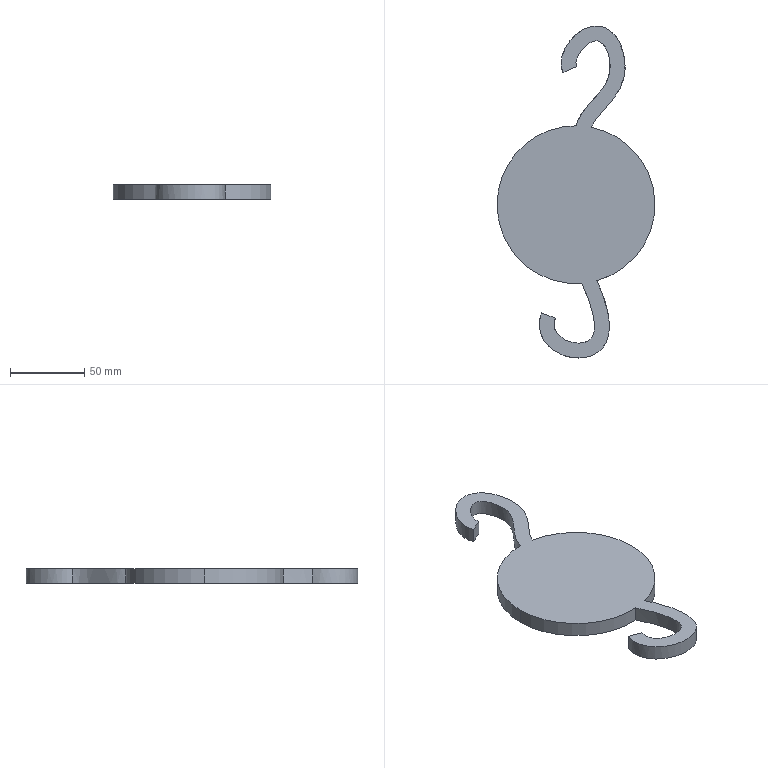Part | STEP file | Spring scale | 1 solid | 11 faces | box 106.116 x 223.189 x 10 mm | volume 107592 mm3 | plane 4 | spline 4 | cylinder 3 | commonest cylinder face diameters 106.116 x3
STEP:
#1=CARTESIAN_POINT('',(0.,0.,0.));
#2=DIRECTION('',(0.,0.,1.));
#3=DIRECTION('',(1.,0.,0.));
#4=AXIS2_PLACEMENT_3D('',#1,#2,#3);
#5=CARTESIAN_POINT('',(-53.422,-92.835,10.));
#6=VERTEX_POINT('',#5);
#7=CARTESIAN_POINT('',(3.465,-145.754,10.));
#8=VERTEX_POINT('',#7);
#9=CARTESIAN_POINT('',(-0.3636,-92.835,10.));
#10=DIRECTION('',(0.,0.,1.));
#11=DIRECTION('',(-1.,0.,0.));
#12=AXIS2_PLACEMENT_3D('',#9,#10,#11);
#13=CIRCLE('',#12,53.058);
#14=CARTESIAN_POINT('',(-0.3636,-92.835,10.));
#15=DIRECTION('',(0.,0.,-1.));
#16=DIRECTION('',(-1.,0.,0.));
#17=AXIS2_PLACEMENT_3D('',#14,#15,#16);
#18=CYLINDRICAL_SURFACE('',#17,53.058);
#19=CARTESIAN_POINT('',(6.283,0.));
#20=DIRECTION('',(-1.,0.));
#21=VECTOR('',#20,1.);
#22=LINE('',#19,#21);
#23=(GEOMETRIC_REPRESENTATION_CONTEXT(2)PARAMETRIC_REPRESENTATION_CONTEXT()REPRESENTATION_CONTEXT('',''));
#24=DEFINITIONAL_REPRESENTATION('',(#22),#23);
#25=PCURVE('',#18,#24);
#26=CARTESIAN_POINT('',(22.563,-1.634,10.));
#27=DIRECTION('',(0.,0.,1.));
#28=DIRECTION('',(1.,0.,0.));
#29=AXIS2_PLACEMENT_3D('',#26,#27,#28);
#30=PLANE('',#29);
#31=CARTESIAN_POINT('',(-22.927,-91.2));
#32=DIRECTION('',(-1.,0.));
#33=AXIS2_PLACEMENT_2D('',#31,#32);
#34=CIRCLE('',#33,53.058);
#35=(GEOMETRIC_REPRESENTATION_CONTEXT(2)PARAMETRIC_REPRESENTATION_CONTEXT()REPRESENTATION_CONTEXT('',''));
#36=DEFINITIONAL_REPRESENTATION('',(#34),#35);
#37=PCURVE('',#30,#36);
#38=SURFACE_CURVE('',#13,(#25,#37),.PCURVE_S1.);
#39=EDGE_CURVE('',#6,#8,#38,.T.);
#40=ORIENTED_EDGE('',*,*,#39,.F.);
#41=CARTESIAN_POINT('',(-53.422,-92.835,0.));
#42=VERTEX_POINT('',#41);
#43=CARTESIAN_POINT('',(-53.422,-92.835,10.));
#44=DIRECTION('',(0.,0.,-1.));
#45=VECTOR('',#44,1.);
#46=LINE('',#43,#45);
#47=CARTESIAN_POINT('',(6.283,0.));
#48=DIRECTION('',(0.,1.));
#49=VECTOR('',#48,1.);
#50=LINE('',#47,#49);
#51=(GEOMETRIC_REPRESENTATION_CONTEXT(2)PARAMETRIC_REPRESENTATION_CONTEXT()REPRESENTATION_CONTEXT('',''));
#52=DEFINITIONAL_REPRESENTATION('',(#50),#51);
#53=PCURVE('',#18,#52);
#54=CARTESIAN_POINT('',(-0.3636,-92.835,10.));
#55=DIRECTION('',(0.,0.,-1.));
#56=DIRECTION('',(-1.,0.,0.));
#57=AXIS2_PLACEMENT_3D('',#54,#55,#56);
#58=CYLINDRICAL_SURFACE('',#57,53.058);
#59=CARTESIAN_POINT('',(0.,0.));
#60=DIRECTION('',(0.,1.));
#61=VECTOR('',#60,1.);
#62=LINE('',#59,#61);
#63=(GEOMETRIC_REPRESENTATION_CONTEXT(2)PARAMETRIC_REPRESENTATION_CONTEXT()REPRESENTATION_CONTEXT('',''));
#64=DEFINITIONAL_REPRESENTATION('',(#62),#63);
#65=PCURVE('',#58,#64);
#66=SURFACE_CURVE('',#46,(#53,#65),.PCURVE_S1.);
#67=EDGE_CURVE('',#6,#42,#66,.T.);
#68=ORIENTED_EDGE('',*,*,#67,.T.);
#69=CARTESIAN_POINT('',(3.465,-145.754,0.));
#70=VERTEX_POINT('',#69);
#71=CARTESIAN_POINT('',(-0.3636,-92.835,0.));
#72=DIRECTION('',(0.,0.,1.));
#73=DIRECTION('',(-1.,0.,0.));
#74=AXIS2_PLACEMENT_3D('',#71,#72,#73);
#75=CIRCLE('',#74,53.058);
#76=CARTESIAN_POINT('',(6.283,10.));
#77=DIRECTION('',(-1.,0.));
#78=VECTOR('',#77,1.);
#79=LINE('',#76,#78);
#80=(GEOMETRIC_REPRESENTATION_CONTEXT(2)PARAMETRIC_REPRESENTATION_CONTEXT()REPRESENTATION_CONTEXT('',''));
#81=DEFINITIONAL_REPRESENTATION('',(#79),#80);
#82=PCURVE('',#18,#81);
#83=CARTESIAN_POINT('',(22.563,-1.634,0.));
#84=DIRECTION('',(0.,0.,1.));
#85=DIRECTION('',(1.,0.,0.));
#86=AXIS2_PLACEMENT_3D('',#83,#84,#85);
#87=PLANE('',#86);
#88=CARTESIAN_POINT('',(-22.927,-91.2));
#89=DIRECTION('',(-1.,0.));
#90=AXIS2_PLACEMENT_2D('',#88,#89);
#91=CIRCLE('',#90,53.058);
#92=(GEOMETRIC_REPRESENTATION_CONTEXT(2)PARAMETRIC_REPRESENTATION_CONTEXT()REPRESENTATION_CONTEXT('',''));
#93=DEFINITIONAL_REPRESENTATION('',(#91),#92);
#94=PCURVE('',#87,#93);
#95=SURFACE_CURVE('',#75,(#82,#94),.PCURVE_S1.);
#96=EDGE_CURVE('',#42,#70,#95,.T.);
#97=ORIENTED_EDGE('',*,*,#96,.T.);
#98=CARTESIAN_POINT('',(3.465,-145.754,5.));
#99=DIRECTION('',(0.,0.,1.));
#100=VECTOR('',#99,1.);
#101=LINE('',#98,#100);
#102=CARTESIAN_POINT('',(4.64,5.));
#103=DIRECTION('',(0.,-1.));
#104=VECTOR('',#103,1.);
#105=LINE('',#102,#104);
#106=(GEOMETRIC_REPRESENTATION_CONTEXT(2)PARAMETRIC_REPRESENTATION_CONTEXT()REPRESENTATION_CONTEXT('',''));
#107=DEFINITIONAL_REPRESENTATION('',(#105),#106);
#108=PCURVE('',#18,#107);
#109=CARTESIAN_POINT('',(3.465,-145.754,10.));
#110=CARTESIAN_POINT('',(3.465,-145.754,0.));
#111=CARTESIAN_POINT('',(3.905,-146.754,10.));
#112=CARTESIAN_POINT('',(3.905,-146.754,0.));
#113=CARTESIAN_POINT('',(6.76,-153.123,10.));
#114=CARTESIAN_POINT('',(6.76,-153.123,0.));
#115=CARTESIAN_POINT('',(11.768,-164.41,10.));
#116=CARTESIAN_POINT('',(11.768,-164.41,0.));
#117=CARTESIAN_POINT('',(14.007,-193.617,10.));
#118=CARTESIAN_POINT('',(14.007,-193.617,0.));
#119=CARTESIAN_POINT('',(-19.503,-183.153,10.));
#120=CARTESIAN_POINT('',(-19.503,-183.153,0.));
#121=CARTESIAN_POINT('',(-14.276,-169.124,10.));
#122=CARTESIAN_POINT('',(-14.276,-169.124,0.));
#123=B_SPLINE_SURFACE_WITH_KNOTS('',3,1,((#109,#110),(#111,#112),(#113,#114),(#115,#116),(#117,#118),(#119,#120),(#121,#122)),.UNSPECIFIED.,.F.,.F.,.F.,(4,1,1,1,4),(2,2),(0.1276,0.1688,0.393,0.6051,1.),(0.,1.),.UNSPECIFIED.);
#124=CARTESIAN_POINT('',(0.1276,1.));
#125=CARTESIAN_POINT('',(0.1276,0.));
#126=B_SPLINE_CURVE_WITH_KNOTS('',1,(#124,#125),.UNSPECIFIED.,.F.,.F.,(2,2),(-5.,5.),.PIECEWISE_BEZIER_KNOTS.);
#127=(GEOMETRIC_REPRESENTATION_CONTEXT(2)PARAMETRIC_REPRESENTATION_CONTEXT()REPRESENTATION_CONTEXT('',''));
#128=DEFINITIONAL_REPRESENTATION('',(#126),#127);
#129=PCURVE('',#123,#128);
#130=SURFACE_CURVE('',#101,(#108,#129),.PCURVE_S1.);
#131=EDGE_CURVE('',#70,#8,#130,.T.);
#132=ORIENTED_EDGE('',*,*,#131,.T.);
#133=EDGE_LOOP('',(#40,#68,#97,#132));
#134=FACE_BOUND('',#133,.T.);
#135=ADVANCED_FACE('',(#134),#18,.T.);
#136=CARTESIAN_POINT('',(9.947,-40.788,10.));
#137=VERTEX_POINT('',#136);
#138=CARTESIAN_POINT('',(-9.171,-3.986,10.));
#139=VERTEX_POINT('',#138);
#140=CARTESIAN_POINT('',(9.947,-40.788,10.));
#141=CARTESIAN_POINT('',(9.973,-40.716,10.));
#142=CARTESIAN_POINT('',(10.186,-40.135,10.));
#143=CARTESIAN_POINT('',(10.896,-38.523,10.));
#144=CARTESIAN_POINT('',(12.625,-35.777,10.));
#145=CARTESIAN_POINT('',(15.676,-32.099,10.));
#146=CARTESIAN_POINT('',(19.453,-28.011,10.));
#147=CARTESIAN_POINT('',(23.604,-23.334,10.));
#148=CARTESIAN_POINT('',(27.701,-17.742,10.));
#149=CARTESIAN_POINT('',(31.119,-10.826,10.));
#150=CARTESIAN_POINT('',(32.629,-3.898,10.));
#151=CARTESIAN_POINT('',(32.657,2.114,10.));
#152=CARTESIAN_POINT('',(32.128,6.58,10.));
#153=CARTESIAN_POINT('',(31.095,11.,10.));
#154=CARTESIAN_POINT('',(29.509,15.321,10.));
#155=CARTESIAN_POINT('',(27.223,19.502,10.));
#156=CARTESIAN_POINT('',(24.407,22.836,10.));
#157=CARTESIAN_POINT('',(21.236,25.171,10.));
#158=CARTESIAN_POINT('',(18.804,26.334,10.));
#159=CARTESIAN_POINT('',(16.636,26.962,10.));
#160=CARTESIAN_POINT('',(14.328,27.351,10.));
#161=CARTESIAN_POINT('',(11.527,27.321,10.));
#162=CARTESIAN_POINT('',(8.59,26.717,10.));
#163=CARTESIAN_POINT('',(5.149,25.439,10.));
#164=CARTESIAN_POINT('',(1.56,23.266,10.));
#165=CARTESIAN_POINT('',(-2.066,20.114,10.));
#166=CARTESIAN_POINT('',(-5.162,16.517,10.));
#167=CARTESIAN_POINT('',(-7.732,12.507,10.));
#168=CARTESIAN_POINT('',(-9.364,8.756,10.));
#169=CARTESIAN_POINT('',(-10.205,5.348,10.));
#170=CARTESIAN_POINT('',(-10.504,2.526,10.));
#171=CARTESIAN_POINT('',(-10.332,-0.09537,10.));
#172=CARTESIAN_POINT('',(-9.821,-2.3,10.));
#173=CARTESIAN_POINT('',(-9.408,-3.44,10.));
#174=CARTESIAN_POINT('',(-9.171,-3.986,10.));
#175=B_SPLINE_CURVE_WITH_KNOTS('',3,(#140,#141,#142,#143,#144,#145,#146,#147,#148,#149,#150,#151,#152,#153,#154,#155,#156,#157,#158,#159,#160,#161,#162,#163,#164,#165,#166,#167,#168,#169,#170,#171,#172,#173,#174),.UNSPECIFIED.,.F.,.F.,(4,1,1,1,1,1,1,1,1,1,1,1,1,1,1,1,1,1,1,1,1,1,1,1,1,1,1,1,1,1,1,1,4),(0.,0.0005756,0.004611,0.01268,0.02075,0.02883,0.0369,0.04497,0.05304,0.06111,0.06515,0.06919,0.07322,0.07726,0.08129,0.08533,0.08735,0.08936,0.09037,0.09138,0.0934,0.09542,0.09744,0.1015,0.1055,0.1095,0.1136,0.1176,0.1196,0.1217,0.1237,0.1247,0.1257),.UNSPECIFIED.);
#176=CARTESIAN_POINT('',(-12.616,-39.154));
#177=CARTESIAN_POINT('',(-12.59,-39.082));
#178=CARTESIAN_POINT('',(-12.378,-38.501));
#179=CARTESIAN_POINT('',(-11.667,-36.889));
#180=CARTESIAN_POINT('',(-9.938,-34.143));
#181=CARTESIAN_POINT('',(-6.887,-30.465));
#182=CARTESIAN_POINT('',(-3.11,-26.376));
#183=CARTESIAN_POINT('',(1.04,-21.7));
#184=CARTESIAN_POINT('',(5.137,-16.108));
#185=CARTESIAN_POINT('',(8.556,-9.191));
#186=CARTESIAN_POINT('',(10.065,-2.264));
#187=CARTESIAN_POINT('',(10.093,3.749));
#188=CARTESIAN_POINT('',(9.565,8.214));
#189=CARTESIAN_POINT('',(8.532,12.635));
#190=CARTESIAN_POINT('',(6.946,16.955));
#191=CARTESIAN_POINT('',(4.66,21.136));
#192=CARTESIAN_POINT('',(1.844,24.47));
#193=CARTESIAN_POINT('',(-1.328,26.806));
#194=CARTESIAN_POINT('',(-3.759,27.969));
#195=CARTESIAN_POINT('',(-5.927,28.596));
#196=CARTESIAN_POINT('',(-8.235,28.985));
#197=CARTESIAN_POINT('',(-11.036,28.955));
#198=CARTESIAN_POINT('',(-13.973,28.351));
#199=CARTESIAN_POINT('',(-17.415,27.073));
#200=CARTESIAN_POINT('',(-21.003,24.9));
#201=CARTESIAN_POINT('',(-24.629,21.749));
#202=CARTESIAN_POINT('',(-27.726,18.151));
#203=CARTESIAN_POINT('',(-30.296,14.141));
#204=CARTESIAN_POINT('',(-31.927,10.39));
#205=CARTESIAN_POINT('',(-32.768,6.983));
#206=CARTESIAN_POINT('',(-33.067,4.16));
#207=CARTESIAN_POINT('',(-32.895,1.539));
#208=CARTESIAN_POINT('',(-32.384,-0.6653));
#209=CARTESIAN_POINT('',(-31.972,-1.806));
#210=CARTESIAN_POINT('',(-31.735,-2.351));
#211=B_SPLINE_CURVE_WITH_KNOTS('',3,(#176,#177,#178,#179,#180,#181,#182,#183,#184,#185,#186,#187,#188,#189,#190,#191,#192,#193,#194,#195,#196,#197,#198,#199,#200,#201,#202,#203,#204,#205,#206,#207,#208,#209,#210),.UNSPECIFIED.,.F.,.F.,(4,1,1,1,1,1,1,1,1,1,1,1,1,1,1,1,1,1,1,1,1,1,1,1,1,1,1,1,1,1,1,1,4),(0.,0.0005756,0.004611,0.01268,0.02075,0.02883,0.0369,0.04497,0.05304,0.06111,0.06515,0.06919,0.07322,0.07726,0.08129,0.08533,0.08735,0.08936,0.09037,0.09138,0.0934,0.09542,0.09744,0.1015,0.1055,0.1095,0.1136,0.1176,0.1196,0.1217,0.1237,0.1247,0.1257),.UNSPECIFIED.);
#212=(GEOMETRIC_REPRESENTATION_CONTEXT(2)PARAMETRIC_REPRESENTATION_CONTEXT()REPRESENTATION_CONTEXT('',''));
#213=DEFINITIONAL_REPRESENTATION('',(#211),#212);
#214=PCURVE('',#30,#213);
#215=CARTESIAN_POINT('',(9.947,-40.788,10.));
#216=CARTESIAN_POINT('',(9.947,-40.788,0.));
#217=CARTESIAN_POINT('',(9.973,-40.716,10.));
#218=CARTESIAN_POINT('',(9.973,-40.716,0.));
#219=CARTESIAN_POINT('',(10.186,-40.135,10.));
#220=CARTESIAN_POINT('',(10.186,-40.135,0.));
#221=CARTESIAN_POINT('',(10.896,-38.523,10.));
#222=CARTESIAN_POINT('',(10.896,-38.523,0.));
#223=CARTESIAN_POINT('',(12.625,-35.777,10.));
#224=CARTESIAN_POINT('',(12.625,-35.777,0.));
#225=CARTESIAN_POINT('',(15.676,-32.099,10.));
#226=CARTESIAN_POINT('',(15.676,-32.099,0.));
#227=CARTESIAN_POINT('',(19.453,-28.011,10.));
#228=CARTESIAN_POINT('',(19.453,-28.011,0.));
#229=CARTESIAN_POINT('',(23.604,-23.334,10.));
#230=CARTESIAN_POINT('',(23.604,-23.334,0.));
#231=CARTESIAN_POINT('',(27.701,-17.742,10.));
#232=CARTESIAN_POINT('',(27.701,-17.742,0.));
#233=CARTESIAN_POINT('',(31.119,-10.826,10.));
#234=CARTESIAN_POINT('',(31.119,-10.826,0.));
#235=CARTESIAN_POINT('',(32.629,-3.898,10.));
#236=CARTESIAN_POINT('',(32.629,-3.898,0.));
#237=CARTESIAN_POINT('',(32.657,2.114,10.));
#238=CARTESIAN_POINT('',(32.657,2.114,0.));
#239=CARTESIAN_POINT('',(32.128,6.58,10.));
#240=CARTESIAN_POINT('',(32.128,6.58,0.));
#241=CARTESIAN_POINT('',(31.095,11.,10.));
#242=CARTESIAN_POINT('',(31.095,11.,0.));
#243=CARTESIAN_POINT('',(29.509,15.321,10.));
#244=CARTESIAN_POINT('',(29.509,15.321,0.));
#245=CARTESIAN_POINT('',(27.223,19.502,10.));
#246=CARTESIAN_POINT('',(27.223,19.502,0.));
#247=CARTESIAN_POINT('',(24.407,22.836,10.));
#248=CARTESIAN_POINT('',(24.407,22.836,0.));
#249=CARTESIAN_POINT('',(21.236,25.171,10.));
#250=CARTESIAN_POINT('',(21.236,25.171,0.));
#251=CARTESIAN_POINT('',(18.804,26.334,10.));
#252=CARTESIAN_POINT('',(18.804,26.334,0.));
#253=CARTESIAN_POINT('',(16.636,26.962,10.));
#254=CARTESIAN_POINT('',(16.636,26.962,0.));
#255=CARTESIAN_POINT('',(14.328,27.351,10.));
#256=CARTESIAN_POINT('',(14.328,27.351,0.));
#257=CARTESIAN_POINT('',(11.527,27.321,10.));
#258=CARTESIAN_POINT('',(11.527,27.321,0.));
#259=CARTESIAN_POINT('',(8.59,26.717,10.));
#260=CARTESIAN_POINT('',(8.59,26.717,0.));
#261=CARTESIAN_POINT('',(5.149,25.439,10.));
#262=CARTESIAN_POINT('',(5.149,25.439,0.));
#263=CARTESIAN_POINT('',(1.56,23.266,10.));
#264=CARTESIAN_POINT('',(1.56,23.266,0.));
#265=CARTESIAN_POINT('',(-2.066,20.114,10.));
#266=CARTESIAN_POINT('',(-2.066,20.114,0.));
#267=CARTESIAN_POINT('',(-5.162,16.517,10.));
#268=CARTESIAN_POINT('',(-5.162,16.517,0.));
#269=CARTESIAN_POINT('',(-7.732,12.507,10.));
#270=CARTESIAN_POINT('',(-7.732,12.507,0.));
#271=CARTESIAN_POINT('',(-9.364,8.756,10.));
#272=CARTESIAN_POINT('',(-9.364,8.756,0.));
#273=CARTESIAN_POINT('',(-10.205,5.348,10.));
#274=CARTESIAN_POINT('',(-10.205,5.348,0.));
#275=CARTESIAN_POINT('',(-10.504,2.526,10.));
#276=CARTESIAN_POINT('',(-10.504,2.526,0.));
#277=CARTESIAN_POINT('',(-10.332,-0.09537,10.));
#278=CARTESIAN_POINT('',(-10.332,-0.09537,0.));
#279=CARTESIAN_POINT('',(-9.821,-2.3,10.));
#280=CARTESIAN_POINT('',(-9.821,-2.3,0.));
#281=CARTESIAN_POINT('',(-9.408,-3.44,10.));
#282=CARTESIAN_POINT('',(-9.408,-3.44,0.));
#283=CARTESIAN_POINT('',(-9.171,-3.986,10.));
#284=CARTESIAN_POINT('',(-9.171,-3.986,0.));
#285=B_SPLINE_SURFACE_WITH_KNOTS('',3,1,((#215,#216),(#217,#218),(#219,#220),(#221,#222),(#223,#224),(#225,#226),(#227,#228),(#229,#230),(#231,#232),(#233,#234),(#235,#236),(#237,#238),(#239,#240),(#241,#242),(#243,#244),(#245,#246),(#247,#248),(#249,#250),(#251,#252),(#253,#254),(#255,#256),(#257,#258),(#259,#260),(#261,#262),(#263,#264),(#265,#266),(#267,#268),(#269,#270),(#271,#272),(#273,#274),(#275,#276),(#277,#278),(#279,#280),(#281,#282),(#283,#284)),.UNSPECIFIED.,.F.,.F.,.F.,(4,1,1,1,1,1,1,1,1,1,1,1,1,1,1,1,1,1,1,1,1,1,1,1,1,1,1,1,1,1,1,1,4),(2,2),(0.02438,0.02843,0.05686,0.1137,0.1706,0.2275,0.2843,0.3412,0.3981,0.4549,0.4833,0.5118,0.5402,0.5686,0.5971,0.6255,0.6397,0.6539,0.6611,0.6682,0.6824,0.6966,0.7108,0.7392,0.7677,0.7961,0.8245,0.853,0.8672,0.8814,0.8956,0.9027,0.9098),(0.,1.),.UNSPECIFIED.);
#286=CARTESIAN_POINT('',(0.02438,0.));
#287=CARTESIAN_POINT('',(0.9098,0.));
#288=B_SPLINE_CURVE_WITH_KNOTS('',1,(#286,#287),.UNSPECIFIED.,.F.,.F.,(2,2),(0.,0.1257),.PIECEWISE_BEZIER_KNOTS.);
#289=(GEOMETRIC_REPRESENTATION_CONTEXT(2)PARAMETRIC_REPRESENTATION_CONTEXT()REPRESENTATION_CONTEXT('',''));
#290=DEFINITIONAL_REPRESENTATION('',(#288),#289);
#291=PCURVE('',#285,#290);
#292=SURFACE_CURVE('',#175,(#214,#291),.PCURVE_S1.);
#293=EDGE_CURVE('',#137,#139,#292,.T.);
#294=ORIENTED_EDGE('',*,*,#293,.T.);
#295=CARTESIAN_POINT('',(0.,0.,10.));
#296=VERTEX_POINT('',#295);
#297=CARTESIAN_POINT('',(-9.171,-3.986,10.));
#298=DIRECTION('',(0.9171,0.3986,0.));
#299=VECTOR('',#298,1.);
#300=LINE('',#297,#299);
#301=CARTESIAN_POINT('',(-31.735,-2.351));
#302=DIRECTION('',(0.9171,0.3986));
#303=VECTOR('',#302,1.);
#304=LINE('',#301,#303);
#305=(GEOMETRIC_REPRESENTATION_CONTEXT(2)PARAMETRIC_REPRESENTATION_CONTEXT()REPRESENTATION_CONTEXT('',''));
#306=DEFINITIONAL_REPRESENTATION('',(#304),#305);
#307=PCURVE('',#30,#306);
#308=CARTESIAN_POINT('',(0.,0.,10.));
#309=DIRECTION('',(-0.3986,0.9171,0.));
#310=DIRECTION('',(-0.9171,-0.3986,0.));
#311=AXIS2_PLACEMENT_3D('',#308,#309,#310);
#312=PLANE('',#311);
#313=CARTESIAN_POINT('',(10.,0.));
#314=DIRECTION('',(-1.,0.));
#315=VECTOR('',#314,1.);
#316=LINE('',#313,#315);
#317=(GEOMETRIC_REPRESENTATION_CONTEXT(2)PARAMETRIC_REPRESENTATION_CONTEXT()REPRESENTATION_CONTEXT('',''));
#318=DEFINITIONAL_REPRESENTATION('',(#316),#317);
#319=PCURVE('',#312,#318);
#320=SURFACE_CURVE('',#300,(#307,#319),.PCURVE_S1.);
#321=EDGE_CURVE('',#139,#296,#320,.T.);
#322=ORIENTED_EDGE('',*,*,#321,.T.);
#323=CARTESIAN_POINT('',(-0.1695,-39.777,10.));
#324=VERTEX_POINT('',#323);
#325=CARTESIAN_POINT('',(0.,0.,10.));
#326=CARTESIAN_POINT('',(-1.471,3.385,10.));
#327=CARTESIAN_POINT('',(3.016,12.859,10.));
#328=CARTESIAN_POINT('',(17.542,21.493,10.));
#329=CARTESIAN_POINT('',(26.271,-2.671,10.));
#330=CARTESIAN_POINT('',(13.888,-20.608,10.));
#331=CARTESIAN_POINT('',(1.844,-31.366,10.));
#332=CARTESIAN_POINT('',(-0.1695,-39.777,10.));
#333=B_SPLINE_CURVE_WITH_KNOTS('',3,(#325,#326,#327,#328,#329,#330,#331,#332),.UNSPECIFIED.,.F.,.F.,(4,1,1,1,1,4),(0.,0.01404,0.02457,0.04464,0.06638,0.0923),.UNSPECIFIED.);
#334=CARTESIAN_POINT('',(-22.563,1.634));
#335=CARTESIAN_POINT('',(-24.034,5.02));
#336=CARTESIAN_POINT('',(-19.548,14.493));
#337=CARTESIAN_POINT('',(-5.021,23.128));
#338=CARTESIAN_POINT('',(3.708,-1.036));
#339=CARTESIAN_POINT('',(-8.675,-18.974));
#340=CARTESIAN_POINT('',(-20.719,-29.731));
#341=CARTESIAN_POINT('',(-22.733,-38.143));
#342=B_SPLINE_CURVE_WITH_KNOTS('',3,(#334,#335,#336,#337,#338,#339,#340,#341),.UNSPECIFIED.,.F.,.F.,(4,1,1,1,1,4),(0.,0.01404,0.02457,0.04464,0.06638,0.0923),.UNSPECIFIED.);
#343=(GEOMETRIC_REPRESENTATION_CONTEXT(2)PARAMETRIC_REPRESENTATION_CONTEXT()REPRESENTATION_CONTEXT('',''));
#344=DEFINITIONAL_REPRESENTATION('',(#342),#343);
#345=PCURVE('',#30,#344);
#346=CARTESIAN_POINT('',(0.,0.,10.));
#347=CARTESIAN_POINT('',(0.,0.,0.));
#348=CARTESIAN_POINT('',(-1.471,3.385,10.));
#349=CARTESIAN_POINT('',(-1.471,3.385,0.));
#350=CARTESIAN_POINT('',(3.016,12.859,10.));
#351=CARTESIAN_POINT('',(3.016,12.859,0.));
#352=CARTESIAN_POINT('',(17.542,21.493,10.));
#353=CARTESIAN_POINT('',(17.542,21.493,0.));
#354=CARTESIAN_POINT('',(26.271,-2.671,10.));
#355=CARTESIAN_POINT('',(26.271,-2.671,0.));
#356=CARTESIAN_POINT('',(13.888,-20.608,10.));
#357=CARTESIAN_POINT('',(13.888,-20.608,0.));
#358=CARTESIAN_POINT('',(1.844,-31.366,10.));
#359=CARTESIAN_POINT('',(1.844,-31.366,0.));
#360=CARTESIAN_POINT('',(-0.1695,-39.777,10.));
#361=CARTESIAN_POINT('',(-0.1695,-39.777,0.));
#362=B_SPLINE_SURFACE_WITH_KNOTS('',3,1,((#346,#347),(#348,#349),(#350,#351),(#352,#353),(#354,#355),(#356,#357),(#358,#359),(#360,#361)),.UNSPECIFIED.,.F.,.F.,.F.,(4,1,1,1,1,4),(2,2),(0.,0.1384,0.2422,0.44,0.6543,0.9098),(0.,1.),.UNSPECIFIED.);
#363=CARTESIAN_POINT('',(0.,0.));
#364=CARTESIAN_POINT('',(0.9098,0.));
#365=B_SPLINE_CURVE_WITH_KNOTS('',1,(#363,#364),.UNSPECIFIED.,.F.,.F.,(2,2),(0.,0.0923),.PIECEWISE_BEZIER_KNOTS.);
#366=(GEOMETRIC_REPRESENTATION_CONTEXT(2)PARAMETRIC_REPRESENTATION_CONTEXT()REPRESENTATION_CONTEXT('',''));
#367=DEFINITIONAL_REPRESENTATION('',(#365),#366);
#368=PCURVE('',#362,#367);
#369=SURFACE_CURVE('',#333,(#345,#368),.PCURVE_S1.);
#370=EDGE_CURVE('',#296,#324,#369,.T.);
#371=ORIENTED_EDGE('',*,*,#370,.T.);
#372=CARTESIAN_POINT('',(-0.3636,-92.835,10.));
#373=DIRECTION('',(0.,0.,1.));
#374=DIRECTION('',(-1.,0.,0.));
#375=AXIS2_PLACEMENT_3D('',#372,#373,#374);
#376=CIRCLE('',#375,53.058);
#377=CARTESIAN_POINT('',(-22.927,-91.2));
#378=DIRECTION('',(-1.,0.));
#379=AXIS2_PLACEMENT_2D('',#377,#378);
#380=CIRCLE('',#379,53.058);
#381=(GEOMETRIC_REPRESENTATION_CONTEXT(2)PARAMETRIC_REPRESENTATION_CONTEXT()REPRESENTATION_CONTEXT('',''));
#382=DEFINITIONAL_REPRESENTATION('',(#380),#381);
#383=PCURVE('',#30,#382);
#384=CARTESIAN_POINT('',(6.283,0.));
#385=DIRECTION('',(-1.,0.));
#386=VECTOR('',#385,1.);
#387=LINE('',#384,#386);
#388=(GEOMETRIC_REPRESENTATION_CONTEXT(2)PARAMETRIC_REPRESENTATION_CONTEXT()REPRESENTATION_CONTEXT('',''));
#389=DEFINITIONAL_REPRESENTATION('',(#387),#388);
#390=PCURVE('',#58,#389);
#391=SURFACE_CURVE('',#376,(#383,#390),.PCURVE_S1.);
#392=EDGE_CURVE('',#324,#6,#391,.T.);
#393=ORIENTED_EDGE('',*,*,#392,.T.);
#394=ORIENTED_EDGE('',*,*,#39,.T.);
#395=CARTESIAN_POINT('',(-14.276,-169.124,10.));
#396=VERTEX_POINT('',#395);
#397=CARTESIAN_POINT('',(3.465,-145.754,10.));
#398=CARTESIAN_POINT('',(3.905,-146.754,10.));
#399=CARTESIAN_POINT('',(6.76,-153.123,10.));
#400=CARTESIAN_POINT('',(11.768,-164.41,10.));
#401=CARTESIAN_POINT('',(14.007,-193.617,10.));
#402=CARTESIAN_POINT('',(-19.503,-183.153,10.));
#403=CARTESIAN_POINT('',(-14.276,-169.124,10.));
#404=B_SPLINE_CURVE_WITH_KNOTS('',3,(#397,#398,#399,#400,#401,#402,#403),.UNSPECIFIED.,.F.,.F.,(4,1,1,1,4),(0.,0.003539,0.0228,0.04103,0.07495),.UNSPECIFIED.);
#405=CARTESIAN_POINT('',(-19.098,-144.12));
#406=CARTESIAN_POINT('',(-18.659,-145.12));
#407=CARTESIAN_POINT('',(-15.804,-151.489));
#408=CARTESIAN_POINT('',(-10.796,-162.776));
#409=CARTESIAN_POINT('',(-8.556,-191.983));
#410=CARTESIAN_POINT('',(-42.067,-181.519));
#411=CARTESIAN_POINT('',(-36.84,-167.49));
#412=B_SPLINE_CURVE_WITH_KNOTS('',3,(#405,#406,#407,#408,#409,#410,#411),.UNSPECIFIED.,.F.,.F.,(4,1,1,1,4),(0.,0.003539,0.0228,0.04103,0.07495),.UNSPECIFIED.);
#413=(GEOMETRIC_REPRESENTATION_CONTEXT(2)PARAMETRIC_REPRESENTATION_CONTEXT()REPRESENTATION_CONTEXT('',''));
#414=DEFINITIONAL_REPRESENTATION('',(#412),#413);
#415=PCURVE('',#30,#414);
#416=CARTESIAN_POINT('',(0.1276,0.));
#417=CARTESIAN_POINT('',(1.,0.));
#418=B_SPLINE_CURVE_WITH_KNOTS('',1,(#416,#417),.UNSPECIFIED.,.F.,.F.,(2,2),(0.,0.07495),.PIECEWISE_BEZIER_KNOTS.);
#419=(GEOMETRIC_REPRESENTATION_CONTEXT(2)PARAMETRIC_REPRESENTATION_CONTEXT()REPRESENTATION_CONTEXT('',''));
#420=DEFINITIONAL_REPRESENTATION('',(#418),#419);
#421=PCURVE('',#123,#420);
#422=SURFACE_CURVE('',#404,(#415,#421),.PCURVE_S1.);
#423=EDGE_CURVE('',#8,#396,#422,.T.);
#424=ORIENTED_EDGE('',*,*,#423,.T.);
#425=CARTESIAN_POINT('',(-23.647,-165.633,10.));
#426=VERTEX_POINT('',#425);
#427=CARTESIAN_POINT('',(-14.276,-169.124,10.));
#428=DIRECTION('',(-0.9371,0.3491,0.));
#429=VECTOR('',#428,1.);
#430=LINE('',#427,#429);
#431=CARTESIAN_POINT('',(-36.84,-167.49));
#432=DIRECTION('',(-0.9371,0.3491));
#433=VECTOR('',#432,1.);
#434=LINE('',#431,#433);
#435=(GEOMETRIC_REPRESENTATION_CONTEXT(2)PARAMETRIC_REPRESENTATION_CONTEXT()REPRESENTATION_CONTEXT('',''));
#436=DEFINITIONAL_REPRESENTATION('',(#434),#435);
#437=PCURVE('',#30,#436);
#438=CARTESIAN_POINT('',(-14.276,-169.124,10.));
#439=DIRECTION('',(-0.3491,-0.9371,0.));
#440=DIRECTION('',(0.9371,-0.3491,0.));
#441=AXIS2_PLACEMENT_3D('',#438,#439,#440);
#442=PLANE('',#441);
#443=CARTESIAN_POINT('',(0.,0.));
#444=DIRECTION('',(-1.,0.));
#445=VECTOR('',#444,1.);
#446=LINE('',#443,#445);
#447=(GEOMETRIC_REPRESENTATION_CONTEXT(2)PARAMETRIC_REPRESENTATION_CONTEXT()REPRESENTATION_CONTEXT('',''));
#448=DEFINITIONAL_REPRESENTATION('',(#446),#447);
#449=PCURVE('',#442,#448);
#450=SURFACE_CURVE('',#430,(#437,#449),.PCURVE_S1.);
#451=EDGE_CURVE('',#396,#426,#450,.T.);
#452=ORIENTED_EDGE('',*,*,#451,.T.);
#453=CARTESIAN_POINT('',(13.634,-144.013,10.));
#454=VERTEX_POINT('',#453);
#455=CARTESIAN_POINT('',(-23.647,-165.633,10.));
#456=CARTESIAN_POINT('',(-24.247,-167.243,10.));
#457=CARTESIAN_POINT('',(-25.114,-170.621,10.));
#458=CARTESIAN_POINT('',(-25.145,-175.755,10.));
#459=CARTESIAN_POINT('',(-23.91,-180.583,10.));
#460=CARTESIAN_POINT('',(-20.93,-186.099,10.));
#461=CARTESIAN_POINT('',(-15.701,-190.994,10.));
#462=CARTESIAN_POINT('',(-8.635,-194.453,10.));
#463=CARTESIAN_POINT('',(-2.421,-195.809,10.));
#464=CARTESIAN_POINT('',(2.672,-195.943,10.));
#465=CARTESIAN_POINT('',(6.556,-195.491,10.));
#466=CARTESIAN_POINT('',(10.504,-194.335,10.));
#467=CARTESIAN_POINT('',(13.775,-192.579,10.));
#468=CARTESIAN_POINT('',(16.241,-190.518,10.));
#469=CARTESIAN_POINT('',(18.384,-188.117,10.));
#470=CARTESIAN_POINT('',(20.235,-184.885,10.));
#471=CARTESIAN_POINT('',(21.448,-181.068,10.));
#472=CARTESIAN_POINT('',(21.99,-177.446,10.));
#473=CARTESIAN_POINT('',(22.095,-174.003,10.));
#474=CARTESIAN_POINT('',(21.833,-169.618,10.));
#475=CARTESIAN_POINT('',(20.986,-164.517,10.));
#476=CARTESIAN_POINT('',(19.148,-157.295,10.));
#477=CARTESIAN_POINT('',(16.759,-151.052,10.));
#478=CARTESIAN_POINT('',(14.698,-146.387,10.));
#479=CARTESIAN_POINT('',(13.87,-144.539,10.));
#480=CARTESIAN_POINT('',(13.634,-144.013,10.));
#481=B_SPLINE_CURVE_WITH_KNOTS('',3,(#455,#456,#457,#458,#459,#460,#461,#462,#463,#464,#465,#466,#467,#468,#469,#470,#471,#472,#473,#474,#475,#476,#477,#478,#479,#480),.UNSPECIFIED.,.F.,.F.,(4,1,1,1,1,1,1,1,1,1,1,1,1,1,1,1,1,1,1,1,1,1,1,4),(0.,0.003613,0.007227,0.01084,0.01445,0.02168,0.02891,0.03613,0.03975,0.04336,0.04698,0.05059,0.0524,0.0542,0.05782,0.06143,0.06504,0.06866,0.07227,0.0795,0.08672,0.1012,0.1084,0.1113),.UNSPECIFIED.);
#482=CARTESIAN_POINT('',(-46.21,-163.999));
#483=CARTESIAN_POINT('',(-46.81,-165.609));
#484=CARTESIAN_POINT('',(-47.677,-168.986));
#485=CARTESIAN_POINT('',(-47.708,-174.121));
#486=CARTESIAN_POINT('',(-46.473,-178.949));
#487=CARTESIAN_POINT('',(-43.493,-184.465));
#488=CARTESIAN_POINT('',(-38.265,-189.36));
#489=CARTESIAN_POINT('',(-31.198,-192.819));
#490=CARTESIAN_POINT('',(-24.984,-194.174));
#491=CARTESIAN_POINT('',(-19.891,-194.309));
#492=CARTESIAN_POINT('',(-16.007,-193.856));
#493=CARTESIAN_POINT('',(-12.059,-192.701));
#494=CARTESIAN_POINT('',(-8.789,-190.945));
#495=CARTESIAN_POINT('',(-6.322,-188.884));
#496=CARTESIAN_POINT('',(-4.179,-186.483));
#497=CARTESIAN_POINT('',(-2.328,-183.25));
#498=CARTESIAN_POINT('',(-1.116,-179.434));
#499=CARTESIAN_POINT('',(-0.5732,-175.812));
#500=CARTESIAN_POINT('',(-0.4686,-172.369));
#501=CARTESIAN_POINT('',(-0.7305,-167.983));
#502=CARTESIAN_POINT('',(-1.577,-162.882));
#503=CARTESIAN_POINT('',(-3.415,-155.661));
#504=CARTESIAN_POINT('',(-5.804,-149.418));
#505=CARTESIAN_POINT('',(-7.865,-144.753));
#506=CARTESIAN_POINT('',(-8.694,-142.905));
#507=CARTESIAN_POINT('',(-8.929,-142.379));
#508=B_SPLINE_CURVE_WITH_KNOTS('',3,(#482,#483,#484,#485,#486,#487,#488,#489,#490,#491,#492,#493,#494,#495,#496,#497,#498,#499,#500,#501,#502,#503,#504,#505,#506,#507),.UNSPECIFIED.,.F.,.F.,(4,1,1,1,1,1,1,1,1,1,1,1,1,1,1,1,1,1,1,1,1,1,1,4),(0.,0.003613,0.007227,0.01084,0.01445,0.02168,0.02891,0.03613,0.03975,0.04336,0.04698,0.05059,0.0524,0.0542,0.05782,0.06143,0.06504,0.06866,0.07227,0.0795,0.08672,0.1012,0.1084,0.1113),.UNSPECIFIED.);
#509=(GEOMETRIC_REPRESENTATION_CONTEXT(2)PARAMETRIC_REPRESENTATION_CONTEXT()REPRESENTATION_CONTEXT('',''));
#510=DEFINITIONAL_REPRESENTATION('',(#508),#509);
#511=PCURVE('',#30,#510);
#512=CARTESIAN_POINT('',(-23.647,-165.633,10.));
#513=CARTESIAN_POINT('',(-23.647,-165.633,0.));
#514=CARTESIAN_POINT('',(-24.247,-167.243,10.));
#515=CARTESIAN_POINT('',(-24.247,-167.243,0.));
#516=CARTESIAN_POINT('',(-25.114,-170.621,10.));
#517=CARTESIAN_POINT('',(-25.114,-170.621,0.));
#518=CARTESIAN_POINT('',(-25.145,-175.755,10.));
#519=CARTESIAN_POINT('',(-25.145,-175.755,0.));
#520=CARTESIAN_POINT('',(-23.91,-180.583,10.));
#521=CARTESIAN_POINT('',(-23.91,-180.583,0.));
#522=CARTESIAN_POINT('',(-20.93,-186.099,10.));
#523=CARTESIAN_POINT('',(-20.93,-186.099,0.));
#524=CARTESIAN_POINT('',(-15.701,-190.994,10.));
#525=CARTESIAN_POINT('',(-15.701,-190.994,0.));
#526=CARTESIAN_POINT('',(-8.635,-194.453,10.));
#527=CARTESIAN_POINT('',(-8.635,-194.453,0.));
#528=CARTESIAN_POINT('',(-2.421,-195.809,10.));
#529=CARTESIAN_POINT('',(-2.421,-195.809,0.));
#530=CARTESIAN_POINT('',(2.672,-195.943,10.));
#531=CARTESIAN_POINT('',(2.672,-195.943,0.));
#532=CARTESIAN_POINT('',(6.556,-195.491,10.));
#533=CARTESIAN_POINT('',(6.556,-195.491,0.));
#534=CARTESIAN_POINT('',(10.504,-194.335,10.));
#535=CARTESIAN_POINT('',(10.504,-194.335,0.));
#536=CARTESIAN_POINT('',(13.775,-192.579,10.));
#537=CARTESIAN_POINT('',(13.775,-192.579,0.));
#538=CARTESIAN_POINT('',(16.241,-190.518,10.));
#539=CARTESIAN_POINT('',(16.241,-190.518,0.));
#540=CARTESIAN_POINT('',(18.384,-188.117,10.));
#541=CARTESIAN_POINT('',(18.384,-188.117,0.));
#542=CARTESIAN_POINT('',(20.235,-184.885,10.));
#543=CARTESIAN_POINT('',(20.235,-184.885,0.));
#544=CARTESIAN_POINT('',(21.448,-181.068,10.));
#545=CARTESIAN_POINT('',(21.448,-181.068,0.));
#546=CARTESIAN_POINT('',(21.99,-177.446,10.));
#547=CARTESIAN_POINT('',(21.99,-177.446,0.));
#548=CARTESIAN_POINT('',(22.095,-174.003,10.));
#549=CARTESIAN_POINT('',(22.095,-174.003,0.));
#550=CARTESIAN_POINT('',(21.833,-169.618,10.));
#551=CARTESIAN_POINT('',(21.833,-169.618,0.));
#552=CARTESIAN_POINT('',(20.986,-164.517,10.));
#553=CARTESIAN_POINT('',(20.986,-164.517,0.));
#554=CARTESIAN_POINT('',(19.148,-157.295,10.));
#555=CARTESIAN_POINT('',(19.148,-157.295,0.));
#556=CARTESIAN_POINT('',(16.759,-151.052,10.));
#557=CARTESIAN_POINT('',(16.759,-151.052,0.));
#558=CARTESIAN_POINT('',(14.698,-146.387,10.));
#559=CARTESIAN_POINT('',(14.698,-146.387,0.));
#560=CARTESIAN_POINT('',(13.87,-144.539,10.));
#561=CARTESIAN_POINT('',(13.87,-144.539,0.));
#562=CARTESIAN_POINT('',(13.634,-144.013,10.));
#563=CARTESIAN_POINT('',(13.634,-144.013,0.));
#564=B_SPLINE_SURFACE_WITH_KNOTS('',3,1,((#512,#513),(#514,#515),(#516,#517),(#518,#519),(#520,#521),(#522,#523),(#524,#525),(#526,#527),(#528,#529),(#530,#531),(#532,#533),(#534,#535),(#536,#537),(#538,#539),(#540,#541),(#542,#543),(#544,#545),(#546,#547),(#548,#549),(#550,#551),(#552,#553),(#554,#555),(#556,#557),(#558,#559),(#560,#561),(#562,#563)),.UNSPECIFIED.,.F.,.F.,.F.,(4,1,1,1,1,1,1,1,1,1,1,1,1,1,1,1,1,1,1,1,1,1,1,4),(2,2),(0.1276,0.1549,0.1821,0.2094,0.2366,0.2912,0.3457,0.4002,0.4275,0.4547,0.482,0.5093,0.5229,0.5365,0.5638,0.5911,0.6183,0.6456,0.6728,0.7274,0.7819,0.8909,0.9455,0.9676),(0.,1.),.UNSPECIFIED.);
#565=CARTESIAN_POINT('',(0.1276,0.));
#566=CARTESIAN_POINT('',(0.9676,0.));
#567=B_SPLINE_CURVE_WITH_KNOTS('',1,(#565,#566),.UNSPECIFIED.,.F.,.F.,(2,2),(0.,0.1113),.PIECEWISE_BEZIER_KNOTS.);
#568=(GEOMETRIC_REPRESENTATION_CONTEXT(2)PARAMETRIC_REPRESENTATION_CONTEXT()REPRESENTATION_CONTEXT('',''));
#569=DEFINITIONAL_REPRESENTATION('',(#567),#568);
#570=PCURVE('',#564,#569);
#571=SURFACE_CURVE('',#481,(#511,#570),.PCURVE_S1.);
#572=EDGE_CURVE('',#426,#454,#571,.T.);
#573=ORIENTED_EDGE('',*,*,#572,.T.);
#574=CARTESIAN_POINT('',(-0.3636,-92.835,10.));
#575=DIRECTION('',(0.,0.,1.));
#576=DIRECTION('',(-1.,0.,0.));
#577=AXIS2_PLACEMENT_3D('',#574,#575,#576);
#578=CIRCLE('',#577,53.058);
#579=CARTESIAN_POINT('',(-22.927,-91.2));
#580=DIRECTION('',(-1.,0.));
#581=AXIS2_PLACEMENT_2D('',#579,#580);
#582=CIRCLE('',#581,53.058);
#583=(GEOMETRIC_REPRESENTATION_CONTEXT(2)PARAMETRIC_REPRESENTATION_CONTEXT()REPRESENTATION_CONTEXT('',''));
#584=DEFINITIONAL_REPRESENTATION('',(#582),#583);
#585=PCURVE('',#30,#584);
#586=CARTESIAN_POINT('',(-0.3636,-92.835,10.));
#587=DIRECTION('',(0.,0.,-1.));
#588=DIRECTION('',(-1.,0.,0.));
#589=AXIS2_PLACEMENT_3D('',#586,#587,#588);
#590=CYLINDRICAL_SURFACE('',#589,53.058);
#591=CARTESIAN_POINT('',(6.283,0.));
#592=DIRECTION('',(-1.,0.));
#593=VECTOR('',#592,1.);
#594=LINE('',#591,#593);
#595=(GEOMETRIC_REPRESENTATION_CONTEXT(2)PARAMETRIC_REPRESENTATION_CONTEXT()REPRESENTATION_CONTEXT('',''));
#596=DEFINITIONAL_REPRESENTATION('',(#594),#595);
#597=PCURVE('',#590,#596);
#598=SURFACE_CURVE('',#578,(#585,#597),.PCURVE_S1.);
#599=EDGE_CURVE('',#454,#137,#598,.T.);
#600=ORIENTED_EDGE('',*,*,#599,.T.);
#601=EDGE_LOOP('',(#294,#322,#371,#393,#394,#424,#452,#573,#600));
#602=FACE_BOUND('',#601,.T.);
#603=ADVANCED_FACE('',(#602),#30,.T.);
#604=CARTESIAN_POINT('',(0.,0.,0.));
#605=VERTEX_POINT('',#604);
#606=CARTESIAN_POINT('',(0.,0.,10.));
#607=DIRECTION('',(0.,0.,-1.));
#608=VECTOR('',#607,1.);
#609=LINE('',#606,#608);
#610=CARTESIAN_POINT('',(0.,0.));
#611=DIRECTION('',(0.,-1.));
#612=VECTOR('',#611,1.);
#613=LINE('',#610,#612);
#614=(GEOMETRIC_REPRESENTATION_CONTEXT(2)PARAMETRIC_REPRESENTATION_CONTEXT()REPRESENTATION_CONTEXT('',''));
#615=DEFINITIONAL_REPRESENTATION('',(#613),#614);
#616=PCURVE('',#312,#615);
#617=CARTESIAN_POINT('',(0.,0.));
#618=CARTESIAN_POINT('',(0.,1.));
#619=B_SPLINE_CURVE_WITH_KNOTS('',1,(#617,#618),.UNSPECIFIED.,.F.,.F.,(2,2),(0.,10.),.PIECEWISE_BEZIER_KNOTS.);
#620=(GEOMETRIC_REPRESENTATION_CONTEXT(2)PARAMETRIC_REPRESENTATION_CONTEXT()REPRESENTATION_CONTEXT('',''));
#621=DEFINITIONAL_REPRESENTATION('',(#619),#620);
#622=PCURVE('',#362,#621);
#623=SURFACE_CURVE('',#609,(#616,#622),.PCURVE_S1.);
#624=EDGE_CURVE('',#296,#605,#623,.T.);
#625=ORIENTED_EDGE('',*,*,#624,.F.);
#626=ORIENTED_EDGE('',*,*,#321,.F.);
#627=CARTESIAN_POINT('',(-9.171,-3.986,0.));
#628=VERTEX_POINT('',#627);
#629=CARTESIAN_POINT('',(-9.171,-3.986,10.));
#630=DIRECTION('',(0.,0.,1.));
#631=VECTOR('',#630,1.);
#632=LINE('',#629,#631);
#633=CARTESIAN_POINT('',(10.,0.));
#634=DIRECTION('',(0.,1.));
#635=VECTOR('',#634,1.);
#636=LINE('',#633,#635);
#637=(GEOMETRIC_REPRESENTATION_CONTEXT(2)PARAMETRIC_REPRESENTATION_CONTEXT()REPRESENTATION_CONTEXT('',''));
#638=DEFINITIONAL_REPRESENTATION('',(#636),#637);
#639=PCURVE('',#312,#638);
#640=CARTESIAN_POINT('',(0.9098,1.));
#641=CARTESIAN_POINT('',(0.9098,0.));
#642=B_SPLINE_CURVE_WITH_KNOTS('',1,(#640,#641),.UNSPECIFIED.,.F.,.F.,(2,2),(-10.,0.),.PIECEWISE_BEZIER_KNOTS.);
#643=(GEOMETRIC_REPRESENTATION_CONTEXT(2)PARAMETRIC_REPRESENTATION_CONTEXT()REPRESENTATION_CONTEXT('',''));
#644=DEFINITIONAL_REPRESENTATION('',(#642),#643);
#645=PCURVE('',#285,#644);
#646=SURFACE_CURVE('',#632,(#639,#645),.PCURVE_S1.);
#647=EDGE_CURVE('',#628,#139,#646,.T.);
#648=ORIENTED_EDGE('',*,*,#647,.F.);
#649=CARTESIAN_POINT('',(0.,0.,0.));
#650=DIRECTION('',(-0.9171,-0.3986,0.));
#651=VECTOR('',#650,1.);
#652=LINE('',#649,#651);
#653=CARTESIAN_POINT('',(0.,-10.));
#654=DIRECTION('',(1.,0.));
#655=VECTOR('',#654,1.);
#656=LINE('',#653,#655);
#657=(GEOMETRIC_REPRESENTATION_CONTEXT(2)PARAMETRIC_REPRESENTATION_CONTEXT()REPRESENTATION_CONTEXT('',''));
#658=DEFINITIONAL_REPRESENTATION('',(#656),#657);
#659=PCURVE('',#312,#658);
#660=CARTESIAN_POINT('',(-22.563,1.634));
#661=DIRECTION('',(-0.9171,-0.3986));
#662=VECTOR('',#661,1.);
#663=LINE('',#660,#662);
#664=(GEOMETRIC_REPRESENTATION_CONTEXT(2)PARAMETRIC_REPRESENTATION_CONTEXT()REPRESENTATION_CONTEXT('',''));
#665=DEFINITIONAL_REPRESENTATION('',(#663),#664);
#666=PCURVE('',#87,#665);
#667=SURFACE_CURVE('',#652,(#659,#666),.PCURVE_S1.);
#668=EDGE_CURVE('',#605,#628,#667,.T.);
#669=ORIENTED_EDGE('',*,*,#668,.F.);
#670=EDGE_LOOP('',(#625,#626,#648,#669));
#671=FACE_BOUND('',#670,.T.);
#672=ADVANCED_FACE('',(#671),#312,.F.);
#673=CARTESIAN_POINT('',(9.947,-40.788,0.));
#674=VERTEX_POINT('',#673);
#675=CARTESIAN_POINT('',(-9.171,-3.986,0.));
#676=CARTESIAN_POINT('',(-9.408,-3.44,0.));
#677=CARTESIAN_POINT('',(-9.821,-2.3,0.));
#678=CARTESIAN_POINT('',(-10.332,-0.09537,0.));
#679=CARTESIAN_POINT('',(-10.504,2.526,0.));
#680=CARTESIAN_POINT('',(-10.205,5.348,0.));
#681=CARTESIAN_POINT('',(-9.364,8.756,0.));
#682=CARTESIAN_POINT('',(-7.732,12.507,0.));
#683=CARTESIAN_POINT('',(-5.162,16.517,0.));
#684=CARTESIAN_POINT('',(-2.066,20.114,0.));
#685=CARTESIAN_POINT('',(1.56,23.266,0.));
#686=CARTESIAN_POINT('',(5.149,25.439,0.));
#687=CARTESIAN_POINT('',(8.59,26.717,0.));
#688=CARTESIAN_POINT('',(11.527,27.321,0.));
#689=CARTESIAN_POINT('',(14.328,27.351,0.));
#690=CARTESIAN_POINT('',(16.636,26.962,0.));
#691=CARTESIAN_POINT('',(18.804,26.334,0.));
#692=CARTESIAN_POINT('',(21.236,25.171,0.));
#693=CARTESIAN_POINT('',(24.407,22.836,0.));
#694=CARTESIAN_POINT('',(27.223,19.502,0.));
#695=CARTESIAN_POINT('',(29.509,15.321,0.));
#696=CARTESIAN_POINT('',(31.095,11.,0.));
#697=CARTESIAN_POINT('',(32.128,6.58,0.));
#698=CARTESIAN_POINT('',(32.657,2.114,0.));
#699=CARTESIAN_POINT('',(32.629,-3.898,0.));
#700=CARTESIAN_POINT('',(31.119,-10.826,0.));
#701=CARTESIAN_POINT('',(27.701,-17.742,0.));
#702=CARTESIAN_POINT('',(23.604,-23.334,0.));
#703=CARTESIAN_POINT('',(19.453,-28.011,0.));
#704=CARTESIAN_POINT('',(15.676,-32.099,0.));
#705=CARTESIAN_POINT('',(12.625,-35.777,0.));
#706=CARTESIAN_POINT('',(10.896,-38.523,0.));
#707=CARTESIAN_POINT('',(10.186,-40.135,0.));
#708=CARTESIAN_POINT('',(9.973,-40.716,0.));
#709=CARTESIAN_POINT('',(9.947,-40.788,0.));
#710=B_SPLINE_CURVE_WITH_KNOTS('',3,(#675,#676,#677,#678,#679,#680,#681,#682,#683,#684,#685,#686,#687,#688,#689,#690,#691,#692,#693,#694,#695,#696,#697,#698,#699,#700,#701,#702,#703,#704,#705,#706,#707,#708,#709),.UNSPECIFIED.,.F.,.F.,(4,1,1,1,1,1,1,1,1,1,1,1,1,1,1,1,1,1,1,1,1,1,1,1,1,1,1,1,1,1,1,1,4),(0.,0.001032,0.002063,0.004126,0.006189,0.008252,0.01238,0.0165,0.02063,0.02476,0.02888,0.03095,0.03301,0.03507,0.0361,0.03714,0.0392,0.04126,0.04539,0.04951,0.05364,0.05777,0.06189,0.06602,0.07427,0.08252,0.09078,0.09903,0.1073,0.1155,0.1238,0.1279,0.1285),.UNSPECIFIED.);
#711=CARTESIAN_POINT('',(0.9098,1.));
#712=CARTESIAN_POINT('',(0.02438,1.));
#713=B_SPLINE_CURVE_WITH_KNOTS('',1,(#711,#712),.UNSPECIFIED.,.F.,.F.,(2,2),(0.,0.1285),.PIECEWISE_BEZIER_KNOTS.);
#714=(GEOMETRIC_REPRESENTATION_CONTEXT(2)PARAMETRIC_REPRESENTATION_CONTEXT()REPRESENTATION_CONTEXT('',''));
#715=DEFINITIONAL_REPRESENTATION('',(#713),#714);
#716=PCURVE('',#285,#715);
#717=CARTESIAN_POINT('',(-31.735,-2.351));
#718=CARTESIAN_POINT('',(-31.972,-1.806));
#719=CARTESIAN_POINT('',(-32.384,-0.6653));
#720=CARTESIAN_POINT('',(-32.895,1.539));
#721=CARTESIAN_POINT('',(-33.067,4.16));
#722=CARTESIAN_POINT('',(-32.768,6.983));
#723=CARTESIAN_POINT('',(-31.927,10.39));
#724=CARTESIAN_POINT('',(-30.296,14.141));
#725=CARTESIAN_POINT('',(-27.726,18.151));
#726=CARTESIAN_POINT('',(-24.629,21.749));
#727=CARTESIAN_POINT('',(-21.003,24.9));
#728=CARTESIAN_POINT('',(-17.415,27.073));
#729=CARTESIAN_POINT('',(-13.973,28.351));
#730=CARTESIAN_POINT('',(-11.036,28.955));
#731=CARTESIAN_POINT('',(-8.235,28.985));
#732=CARTESIAN_POINT('',(-5.927,28.596));
#733=CARTESIAN_POINT('',(-3.759,27.969));
#734=CARTESIAN_POINT('',(-1.328,26.806));
#735=CARTESIAN_POINT('',(1.844,24.47));
#736=CARTESIAN_POINT('',(4.66,21.136));
#737=CARTESIAN_POINT('',(6.946,16.955));
#738=CARTESIAN_POINT('',(8.532,12.635));
#739=CARTESIAN_POINT('',(9.565,8.214));
#740=CARTESIAN_POINT('',(10.093,3.749));
#741=CARTESIAN_POINT('',(10.065,-2.264));
#742=CARTESIAN_POINT('',(8.556,-9.191));
#743=CARTESIAN_POINT('',(5.137,-16.108));
#744=CARTESIAN_POINT('',(1.04,-21.7));
#745=CARTESIAN_POINT('',(-3.11,-26.376));
#746=CARTESIAN_POINT('',(-6.887,-30.465));
#747=CARTESIAN_POINT('',(-9.938,-34.143));
#748=CARTESIAN_POINT('',(-11.667,-36.889));
#749=CARTESIAN_POINT('',(-12.378,-38.501));
#750=CARTESIAN_POINT('',(-12.59,-39.082));
#751=CARTESIAN_POINT('',(-12.616,-39.154));
#752=B_SPLINE_CURVE_WITH_KNOTS('',3,(#717,#718,#719,#720,#721,#722,#723,#724,#725,#726,#727,#728,#729,#730,#731,#732,#733,#734,#735,#736,#737,#738,#739,#740,#741,#742,#743,#744,#745,#746,#747,#748,#749,#750,#751),.UNSPECIFIED.,.F.,.F.,(4,1,1,1,1,1,1,1,1,1,1,1,1,1,1,1,1,1,1,1,1,1,1,1,1,1,1,1,1,1,1,1,4),(0.,0.001032,0.002063,0.004126,0.006189,0.008252,0.01238,0.0165,0.02063,0.02476,0.02888,0.03095,0.03301,0.03507,0.0361,0.03714,0.0392,0.04126,0.04539,0.04951,0.05364,0.05777,0.06189,0.06602,0.07427,0.08252,0.09078,0.09903,0.1073,0.1155,0.1238,0.1279,0.1285),.UNSPECIFIED.);
#753=(GEOMETRIC_REPRESENTATION_CONTEXT(2)PARAMETRIC_REPRESENTATION_CONTEXT()REPRESENTATION_CONTEXT('',''));
#754=DEFINITIONAL_REPRESENTATION('',(#752),#753);
#755=PCURVE('',#87,#754);
#756=SURFACE_CURVE('',#710,(#716,#755),.PCURVE_S1.);
#757=EDGE_CURVE('',#628,#674,#756,.T.);
#758=ORIENTED_EDGE('',*,*,#757,.T.);
#759=CARTESIAN_POINT('',(9.947,-40.788,5.));
#760=DIRECTION('',(0.,0.,1.));
#761=VECTOR('',#760,1.);
#762=LINE('',#759,#761);
#763=CARTESIAN_POINT('',(0.02438,1.));
#764=CARTESIAN_POINT('',(0.02438,0.));
#765=B_SPLINE_CURVE_WITH_KNOTS('',1,(#763,#764),.UNSPECIFIED.,.F.,.F.,(2,2),(-5.,5.),.PIECEWISE_BEZIER_KNOTS.);
#766=(GEOMETRIC_REPRESENTATION_CONTEXT(2)PARAMETRIC_REPRESENTATION_CONTEXT()REPRESENTATION_CONTEXT('',''));
#767=DEFINITIONAL_REPRESENTATION('',(#765),#766);
#768=PCURVE('',#285,#767);
#769=CARTESIAN_POINT('',(1.766,5.));
#770=DIRECTION('',(0.,-1.));
#771=VECTOR('',#770,1.);
#772=LINE('',#769,#771);
#773=(GEOMETRIC_REPRESENTATION_CONTEXT(2)PARAMETRIC_REPRESENTATION_CONTEXT()REPRESENTATION_CONTEXT('',''));
#774=DEFINITIONAL_REPRESENTATION('',(#772),#773);
#775=PCURVE('',#590,#774);
#776=SURFACE_CURVE('',#762,(#768,#775),.PCURVE_S1.);
#777=EDGE_CURVE('',#674,#137,#776,.T.);
#778=ORIENTED_EDGE('',*,*,#777,.T.);
#779=ORIENTED_EDGE('',*,*,#293,.T.);
#780=ORIENTED_EDGE('',*,*,#647,.F.);
#781=EDGE_LOOP('',(#758,#778,#779,#780));
#782=FACE_BOUND('',#781,.F.);
#783=ADVANCED_FACE('',(#782),#285,.F.);
#784=ORIENTED_EDGE('',*,*,#599,.F.);
#785=CARTESIAN_POINT('',(13.634,-144.013,0.));
#786=VERTEX_POINT('',#785);
#787=CARTESIAN_POINT('',(13.634,-144.013,10.));
#788=DIRECTION('',(0.,0.,-1.));
#789=VECTOR('',#788,1.);
#790=LINE('',#787,#789);
#791=CARTESIAN_POINT('',(4.445,0.));
#792=DIRECTION('',(0.,1.));
#793=VECTOR('',#792,1.);
#794=LINE('',#791,#793);
#795=(GEOMETRIC_REPRESENTATION_CONTEXT(2)PARAMETRIC_REPRESENTATION_CONTEXT()REPRESENTATION_CONTEXT('',''));
#796=DEFINITIONAL_REPRESENTATION('',(#794),#795);
#797=PCURVE('',#590,#796);
#798=CARTESIAN_POINT('',(0.9676,0.));
#799=CARTESIAN_POINT('',(0.9676,1.));
#800=B_SPLINE_CURVE_WITH_KNOTS('',1,(#798,#799),.UNSPECIFIED.,.F.,.F.,(2,2),(0.,10.),.PIECEWISE_BEZIER_KNOTS.);
#801=(GEOMETRIC_REPRESENTATION_CONTEXT(2)PARAMETRIC_REPRESENTATION_CONTEXT()REPRESENTATION_CONTEXT('',''));
#802=DEFINITIONAL_REPRESENTATION('',(#800),#801);
#803=PCURVE('',#564,#802);
#804=SURFACE_CURVE('',#790,(#797,#803),.PCURVE_S1.);
#805=EDGE_CURVE('',#454,#786,#804,.T.);
#806=ORIENTED_EDGE('',*,*,#805,.T.);
#807=CARTESIAN_POINT('',(-0.3636,-92.835,0.));
#808=DIRECTION('',(0.,0.,1.));
#809=DIRECTION('',(-1.,0.,0.));
#810=AXIS2_PLACEMENT_3D('',#807,#808,#809);
#811=CIRCLE('',#810,53.058);
#812=CARTESIAN_POINT('',(6.283,10.));
#813=DIRECTION('',(-1.,0.));
#814=VECTOR('',#813,1.);
#815=LINE('',#812,#814);
#816=(GEOMETRIC_REPRESENTATION_CONTEXT(2)PARAMETRIC_REPRESENTATION_CONTEXT()REPRESENTATION_CONTEXT('',''));
#817=DEFINITIONAL_REPRESENTATION('',(#815),#816);
#818=PCURVE('',#590,#817);
#819=CARTESIAN_POINT('',(-22.927,-91.2));
#820=DIRECTION('',(-1.,0.));
#821=AXIS2_PLACEMENT_2D('',#819,#820);
#822=CIRCLE('',#821,53.058);
#823=(GEOMETRIC_REPRESENTATION_CONTEXT(2)PARAMETRIC_REPRESENTATION_CONTEXT()REPRESENTATION_CONTEXT('',''));
#824=DEFINITIONAL_REPRESENTATION('',(#822),#823);
#825=PCURVE('',#87,#824);
#826=SURFACE_CURVE('',#811,(#818,#825),.PCURVE_S1.);
#827=EDGE_CURVE('',#786,#674,#826,.T.);
#828=ORIENTED_EDGE('',*,*,#827,.T.);
#829=ORIENTED_EDGE('',*,*,#777,.T.);
#830=EDGE_LOOP('',(#784,#806,#828,#829));
#831=FACE_BOUND('',#830,.T.);
#832=ADVANCED_FACE('',(#831),#590,.T.);
#833=CARTESIAN_POINT('',(-23.647,-165.633,0.));
#834=VERTEX_POINT('',#833);
#835=CARTESIAN_POINT('',(13.634,-144.013,0.));
#836=CARTESIAN_POINT('',(13.87,-144.539,0.));
#837=CARTESIAN_POINT('',(14.698,-146.387,0.));
#838=CARTESIAN_POINT('',(16.759,-151.052,0.));
#839=CARTESIAN_POINT('',(19.148,-157.295,0.));
#840=CARTESIAN_POINT('',(20.986,-164.517,0.));
#841=CARTESIAN_POINT('',(21.833,-169.618,0.));
#842=CARTESIAN_POINT('',(22.095,-174.003,0.));
#843=CARTESIAN_POINT('',(21.99,-177.446,0.));
#844=CARTESIAN_POINT('',(21.448,-181.068,0.));
#845=CARTESIAN_POINT('',(20.235,-184.885,0.));
#846=CARTESIAN_POINT('',(18.384,-188.117,0.));
#847=CARTESIAN_POINT('',(16.241,-190.518,0.));
#848=CARTESIAN_POINT('',(13.775,-192.579,0.));
#849=CARTESIAN_POINT('',(10.504,-194.335,0.));
#850=CARTESIAN_POINT('',(6.556,-195.491,0.));
#851=CARTESIAN_POINT('',(2.672,-195.943,0.));
#852=CARTESIAN_POINT('',(-2.421,-195.809,0.));
#853=CARTESIAN_POINT('',(-8.635,-194.453,0.));
#854=CARTESIAN_POINT('',(-15.701,-190.994,0.));
#855=CARTESIAN_POINT('',(-20.93,-186.099,0.));
#856=CARTESIAN_POINT('',(-23.91,-180.583,0.));
#857=CARTESIAN_POINT('',(-25.145,-175.755,0.));
#858=CARTESIAN_POINT('',(-25.114,-170.621,0.));
#859=CARTESIAN_POINT('',(-24.247,-167.243,0.));
#860=CARTESIAN_POINT('',(-23.647,-165.633,0.));
#861=B_SPLINE_CURVE_WITH_KNOTS('',3,(#835,#836,#837,#838,#839,#840,#841,#842,#843,#844,#845,#846,#847,#848,#849,#850,#851,#852,#853,#854,#855,#856,#857,#858,#859,#860),.UNSPECIFIED.,.F.,.F.,(4,1,1,1,1,1,1,1,1,1,1,1,1,1,1,1,1,1,1,1,1,1,1,4),(0.,0.002934,0.01017,0.02463,0.03187,0.0391,0.04272,0.04634,0.04995,0.05357,0.05719,0.059,0.0608,0.06442,0.06804,0.07165,0.07527,0.08251,0.08974,0.09697,0.1006,0.1042,0.1078,0.1114),.UNSPECIFIED.);
#862=CARTESIAN_POINT('',(0.9676,1.));
#863=CARTESIAN_POINT('',(0.1276,1.));
#864=B_SPLINE_CURVE_WITH_KNOTS('',1,(#862,#863),.UNSPECIFIED.,.F.,.F.,(2,2),(0.,0.1114),.PIECEWISE_BEZIER_KNOTS.);
#865=(GEOMETRIC_REPRESENTATION_CONTEXT(2)PARAMETRIC_REPRESENTATION_CONTEXT()REPRESENTATION_CONTEXT('',''));
#866=DEFINITIONAL_REPRESENTATION('',(#864),#865);
#867=PCURVE('',#564,#866);
#868=CARTESIAN_POINT('',(-8.929,-142.379));
#869=CARTESIAN_POINT('',(-8.694,-142.905));
#870=CARTESIAN_POINT('',(-7.865,-144.753));
#871=CARTESIAN_POINT('',(-5.804,-149.418));
#872=CARTESIAN_POINT('',(-3.415,-155.661));
#873=CARTESIAN_POINT('',(-1.577,-162.882));
#874=CARTESIAN_POINT('',(-0.7305,-167.983));
#875=CARTESIAN_POINT('',(-0.4686,-172.369));
#876=CARTESIAN_POINT('',(-0.5732,-175.812));
#877=CARTESIAN_POINT('',(-1.116,-179.434));
#878=CARTESIAN_POINT('',(-2.328,-183.25));
#879=CARTESIAN_POINT('',(-4.179,-186.483));
#880=CARTESIAN_POINT('',(-6.322,-188.884));
#881=CARTESIAN_POINT('',(-8.789,-190.945));
#882=CARTESIAN_POINT('',(-12.059,-192.701));
#883=CARTESIAN_POINT('',(-16.007,-193.856));
#884=CARTESIAN_POINT('',(-19.891,-194.309));
#885=CARTESIAN_POINT('',(-24.984,-194.174));
#886=CARTESIAN_POINT('',(-31.198,-192.819));
#887=CARTESIAN_POINT('',(-38.265,-189.36));
#888=CARTESIAN_POINT('',(-43.493,-184.465));
#889=CARTESIAN_POINT('',(-46.473,-178.949));
#890=CARTESIAN_POINT('',(-47.708,-174.121));
#891=CARTESIAN_POINT('',(-47.677,-168.986));
#892=CARTESIAN_POINT('',(-46.81,-165.609));
#893=CARTESIAN_POINT('',(-46.21,-163.999));
#894=B_SPLINE_CURVE_WITH_KNOTS('',3,(#868,#869,#870,#871,#872,#873,#874,#875,#876,#877,#878,#879,#880,#881,#882,#883,#884,#885,#886,#887,#888,#889,#890,#891,#892,#893),.UNSPECIFIED.,.F.,.F.,(4,1,1,1,1,1,1,1,1,1,1,1,1,1,1,1,1,1,1,1,1,1,1,4),(0.,0.002934,0.01017,0.02463,0.03187,0.0391,0.04272,0.04634,0.04995,0.05357,0.05719,0.059,0.0608,0.06442,0.06804,0.07165,0.07527,0.08251,0.08974,0.09697,0.1006,0.1042,0.1078,0.1114),.UNSPECIFIED.);
#895=(GEOMETRIC_REPRESENTATION_CONTEXT(2)PARAMETRIC_REPRESENTATION_CONTEXT()REPRESENTATION_CONTEXT('',''));
#896=DEFINITIONAL_REPRESENTATION('',(#894),#895);
#897=PCURVE('',#87,#896);
#898=SURFACE_CURVE('',#861,(#867,#897),.PCURVE_S1.);
#899=EDGE_CURVE('',#786,#834,#898,.T.);
#900=ORIENTED_EDGE('',*,*,#899,.T.);
#901=CARTESIAN_POINT('',(-23.647,-165.633,5.));
#902=DIRECTION('',(0.,0.,1.));
#903=VECTOR('',#902,1.);
#904=LINE('',#901,#903);
#905=CARTESIAN_POINT('',(0.1276,1.));
#906=CARTESIAN_POINT('',(0.1276,0.));
#907=B_SPLINE_CURVE_WITH_KNOTS('',1,(#905,#906),.UNSPECIFIED.,.F.,.F.,(2,2),(-5.,5.),.PIECEWISE_BEZIER_KNOTS.);
#908=(GEOMETRIC_REPRESENTATION_CONTEXT(2)PARAMETRIC_REPRESENTATION_CONTEXT()REPRESENTATION_CONTEXT('',''));
#909=DEFINITIONAL_REPRESENTATION('',(#907),#908);
#910=PCURVE('',#564,#909);
#911=CARTESIAN_POINT('',(-10.,-5.));
#912=DIRECTION('',(0.,1.));
#913=VECTOR('',#912,1.);
#914=LINE('',#911,#913);
#915=(GEOMETRIC_REPRESENTATION_CONTEXT(2)PARAMETRIC_REPRESENTATION_CONTEXT()REPRESENTATION_CONTEXT('',''));
#916=DEFINITIONAL_REPRESENTATION('',(#914),#915);
#917=PCURVE('',#442,#916);
#918=SURFACE_CURVE('',#904,(#910,#917),.PCURVE_S1.);
#919=EDGE_CURVE('',#834,#426,#918,.T.);
#920=ORIENTED_EDGE('',*,*,#919,.T.);
#921=ORIENTED_EDGE('',*,*,#572,.T.);
#922=ORIENTED_EDGE('',*,*,#805,.T.);
#923=EDGE_LOOP('',(#900,#920,#921,#922));
#924=FACE_BOUND('',#923,.F.);
#925=ADVANCED_FACE('',(#924),#564,.F.);
#926=ORIENTED_EDGE('',*,*,#919,.T.);
#927=ORIENTED_EDGE('',*,*,#451,.F.);
#928=CARTESIAN_POINT('',(-14.276,-169.124,0.));
#929=VERTEX_POINT('',#928);
#930=CARTESIAN_POINT('',(-14.276,-169.124,10.));
#931=DIRECTION('',(0.,0.,1.));
#932=VECTOR('',#931,1.);
#933=LINE('',#930,#932);
#934=CARTESIAN_POINT('',(0.,0.));
#935=DIRECTION('',(0.,1.));
#936=VECTOR('',#935,1.);
#937=LINE('',#934,#936);
#938=(GEOMETRIC_REPRESENTATION_CONTEXT(2)PARAMETRIC_REPRESENTATION_CONTEXT()REPRESENTATION_CONTEXT('',''));
#939=DEFINITIONAL_REPRESENTATION('',(#937),#938);
#940=PCURVE('',#442,#939);
#941=CARTESIAN_POINT('',(1.,1.));
#942=CARTESIAN_POINT('',(1.,0.));
#943=B_SPLINE_CURVE_WITH_KNOTS('',1,(#941,#942),.UNSPECIFIED.,.F.,.F.,(2,2),(-10.,0.),.PIECEWISE_BEZIER_KNOTS.);
#944=(GEOMETRIC_REPRESENTATION_CONTEXT(2)PARAMETRIC_REPRESENTATION_CONTEXT()REPRESENTATION_CONTEXT('',''));
#945=DEFINITIONAL_REPRESENTATION('',(#943),#944);
#946=PCURVE('',#123,#945);
#947=SURFACE_CURVE('',#933,(#940,#946),.PCURVE_S1.);
#948=EDGE_CURVE('',#929,#396,#947,.T.);
#949=ORIENTED_EDGE('',*,*,#948,.F.);
#950=CARTESIAN_POINT('',(-14.276,-169.124,0.));
#951=DIRECTION('',(0.9371,-0.3491,0.));
#952=VECTOR('',#951,1.);
#953=LINE('',#950,#952);
#954=CARTESIAN_POINT('',(0.,-10.));
#955=DIRECTION('',(1.,0.));
#956=VECTOR('',#955,1.);
#957=LINE('',#954,#956);
#958=(GEOMETRIC_REPRESENTATION_CONTEXT(2)PARAMETRIC_REPRESENTATION_CONTEXT()REPRESENTATION_CONTEXT('',''));
#959=DEFINITIONAL_REPRESENTATION('',(#957),#958);
#960=PCURVE('',#442,#959);
#961=CARTESIAN_POINT('',(-36.84,-167.49));
#962=DIRECTION('',(0.9371,-0.3491));
#963=VECTOR('',#962,1.);
#964=LINE('',#961,#963);
#965=(GEOMETRIC_REPRESENTATION_CONTEXT(2)PARAMETRIC_REPRESENTATION_CONTEXT()REPRESENTATION_CONTEXT('',''));
#966=DEFINITIONAL_REPRESENTATION('',(#964),#965);
#967=PCURVE('',#87,#966);
#968=SURFACE_CURVE('',#953,(#960,#967),.PCURVE_S1.);
#969=EDGE_CURVE('',#834,#929,#968,.T.);
#970=ORIENTED_EDGE('',*,*,#969,.F.);
#971=EDGE_LOOP('',(#926,#927,#949,#970));
#972=FACE_BOUND('',#971,.T.);
#973=ADVANCED_FACE('',(#972),#442,.F.);
#974=CARTESIAN_POINT('',(-14.276,-169.124,0.));
#975=CARTESIAN_POINT('',(-19.503,-183.153,0.));
#976=CARTESIAN_POINT('',(14.007,-193.617,0.));
#977=CARTESIAN_POINT('',(11.768,-164.41,0.));
#978=CARTESIAN_POINT('',(6.76,-153.123,0.));
#979=CARTESIAN_POINT('',(3.905,-146.754,0.));
#980=CARTESIAN_POINT('',(3.465,-145.754,0.));
#981=B_SPLINE_CURVE_WITH_KNOTS('',3,(#974,#975,#976,#977,#978,#979,#980),.UNSPECIFIED.,.F.,.F.,(4,1,1,1,4),(0.,0.03408,0.05239,0.07175,0.0753),.UNSPECIFIED.);
#982=CARTESIAN_POINT('',(1.,1.));
#983=CARTESIAN_POINT('',(0.1276,1.));
#984=B_SPLINE_CURVE_WITH_KNOTS('',1,(#982,#983),.UNSPECIFIED.,.F.,.F.,(2,2),(0.,0.0753),.PIECEWISE_BEZIER_KNOTS.);
#985=(GEOMETRIC_REPRESENTATION_CONTEXT(2)PARAMETRIC_REPRESENTATION_CONTEXT()REPRESENTATION_CONTEXT('',''));
#986=DEFINITIONAL_REPRESENTATION('',(#984),#985);
#987=PCURVE('',#123,#986);
#988=CARTESIAN_POINT('',(-36.84,-167.49));
#989=CARTESIAN_POINT('',(-42.067,-181.519));
#990=CARTESIAN_POINT('',(-8.556,-191.983));
#991=CARTESIAN_POINT('',(-10.796,-162.776));
#992=CARTESIAN_POINT('',(-15.804,-151.489));
#993=CARTESIAN_POINT('',(-18.659,-145.12));
#994=CARTESIAN_POINT('',(-19.098,-144.12));
#995=B_SPLINE_CURVE_WITH_KNOTS('',3,(#988,#989,#990,#991,#992,#993,#994),.UNSPECIFIED.,.F.,.F.,(4,1,1,1,4),(0.,0.03408,0.05239,0.07175,0.0753),.UNSPECIFIED.);
#996=(GEOMETRIC_REPRESENTATION_CONTEXT(2)PARAMETRIC_REPRESENTATION_CONTEXT()REPRESENTATION_CONTEXT('',''));
#997=DEFINITIONAL_REPRESENTATION('',(#995),#996);
#998=PCURVE('',#87,#997);
#999=SURFACE_CURVE('',#981,(#987,#998),.PCURVE_S1.);
#1000=EDGE_CURVE('',#929,#70,#999,.T.);
#1001=ORIENTED_EDGE('',*,*,#1000,.T.);
#1002=ORIENTED_EDGE('',*,*,#131,.T.);
#1003=ORIENTED_EDGE('',*,*,#423,.T.);
#1004=ORIENTED_EDGE('',*,*,#948,.F.);
#1005=EDGE_LOOP('',(#1001,#1002,#1003,#1004));
#1006=FACE_BOUND('',#1005,.F.);
#1007=ADVANCED_FACE('',(#1006),#123,.F.);
#1008=ORIENTED_EDGE('',*,*,#67,.F.);
#1009=ORIENTED_EDGE('',*,*,#392,.F.);
#1010=CARTESIAN_POINT('',(-0.1695,-39.777,0.));
#1011=VERTEX_POINT('',#1010);
#1012=CARTESIAN_POINT('',(-0.1695,-39.777,10.));
#1013=DIRECTION('',(0.,0.,-1.));
#1014=VECTOR('',#1013,1.);
#1015=LINE('',#1012,#1014);
#1016=CARTESIAN_POINT('',(1.574,0.));
#1017=DIRECTION('',(0.,1.));
#1018=VECTOR('',#1017,1.);
#1019=LINE('',#1016,#1018);
#1020=(GEOMETRIC_REPRESENTATION_CONTEXT(2)PARAMETRIC_REPRESENTATION_CONTEXT()REPRESENTATION_CONTEXT('',''));
#1021=DEFINITIONAL_REPRESENTATION('',(#1019),#1020);
#1022=PCURVE('',#58,#1021);
#1023=CARTESIAN_POINT('',(0.9098,0.));
#1024=CARTESIAN_POINT('',(0.9098,1.));
#1025=B_SPLINE_CURVE_WITH_KNOTS('',1,(#1023,#1024),.UNSPECIFIED.,.F.,.F.,(2,2),(0.,10.),.PIECEWISE_BEZIER_KNOTS.);
#1026=(GEOMETRIC_REPRESENTATION_CONTEXT(2)PARAMETRIC_REPRESENTATION_CONTEXT()REPRESENTATION_CONTEXT('',''));
#1027=DEFINITIONAL_REPRESENTATION('',(#1025),#1026);
#1028=PCURVE('',#362,#1027);
#1029=SURFACE_CURVE('',#1015,(#1022,#1028),.PCURVE_S1.);
#1030=EDGE_CURVE('',#324,#1011,#1029,.T.);
#1031=ORIENTED_EDGE('',*,*,#1030,.T.);
#1032=CARTESIAN_POINT('',(-0.3636,-92.835,0.));
#1033=DIRECTION('',(0.,0.,1.));
#1034=DIRECTION('',(-1.,0.,0.));
#1035=AXIS2_PLACEMENT_3D('',#1032,#1033,#1034);
#1036=CIRCLE('',#1035,53.058);
#1037=CARTESIAN_POINT('',(6.283,10.));
#1038=DIRECTION('',(-1.,0.));
#1039=VECTOR('',#1038,1.);
#1040=LINE('',#1037,#1039);
#1041=(GEOMETRIC_REPRESENTATION_CONTEXT(2)PARAMETRIC_REPRESENTATION_CONTEXT()REPRESENTATION_CONTEXT('',''));
#1042=DEFINITIONAL_REPRESENTATION('',(#1040),#1041);
#1043=PCURVE('',#58,#1042);
#1044=CARTESIAN_POINT('',(-22.927,-91.2));
#1045=DIRECTION('',(-1.,0.));
#1046=AXIS2_PLACEMENT_2D('',#1044,#1045);
#1047=CIRCLE('',#1046,53.058);
#1048=(GEOMETRIC_REPRESENTATION_CONTEXT(2)PARAMETRIC_REPRESENTATION_CONTEXT()REPRESENTATION_CONTEXT('',''));
#1049=DEFINITIONAL_REPRESENTATION('',(#1047),#1048);
#1050=PCURVE('',#87,#1049);
#1051=SURFACE_CURVE('',#1036,(#1043,#1050),.PCURVE_S1.);
#1052=EDGE_CURVE('',#1011,#42,#1051,.T.);
#1053=ORIENTED_EDGE('',*,*,#1052,.T.);
#1054=EDGE_LOOP('',(#1008,#1009,#1031,#1053));
#1055=FACE_BOUND('',#1054,.T.);
#1056=ADVANCED_FACE('',(#1055),#58,.T.);
#1057=CARTESIAN_POINT('',(-0.1695,-39.777,0.));
#1058=CARTESIAN_POINT('',(1.844,-31.366,0.));
#1059=CARTESIAN_POINT('',(13.888,-20.608,0.));
#1060=CARTESIAN_POINT('',(26.271,-2.671,0.));
#1061=CARTESIAN_POINT('',(17.542,21.493,0.));
#1062=CARTESIAN_POINT('',(3.016,12.859,0.));
#1063=CARTESIAN_POINT('',(-1.471,3.385,0.));
#1064=CARTESIAN_POINT('',(0.,0.,0.));
#1065=B_SPLINE_CURVE_WITH_KNOTS('',3,(#1057,#1058,#1059,#1060,#1061,#1062,#1063,#1064),.UNSPECIFIED.,.F.,.F.,(4,1,1,1,1,4),(0.,0.02578,0.0474,0.06736,0.07783,0.0918),.UNSPECIFIED.);
#1066=CARTESIAN_POINT('',(0.9098,1.));
#1067=CARTESIAN_POINT('',(0.,1.));
#1068=B_SPLINE_CURVE_WITH_KNOTS('',1,(#1066,#1067),.UNSPECIFIED.,.F.,.F.,(2,2),(0.,0.0918),.PIECEWISE_BEZIER_KNOTS.);
#1069=(GEOMETRIC_REPRESENTATION_CONTEXT(2)PARAMETRIC_REPRESENTATION_CONTEXT()REPRESENTATION_CONTEXT('',''));
#1070=DEFINITIONAL_REPRESENTATION('',(#1068),#1069);
#1071=PCURVE('',#362,#1070);
#1072=CARTESIAN_POINT('',(-22.733,-38.143));
#1073=CARTESIAN_POINT('',(-20.719,-29.731));
#1074=CARTESIAN_POINT('',(-8.675,-18.974));
#1075=CARTESIAN_POINT('',(3.708,-1.036));
#1076=CARTESIAN_POINT('',(-5.021,23.128));
#1077=CARTESIAN_POINT('',(-19.548,14.493));
#1078=CARTESIAN_POINT('',(-24.034,5.02));
#1079=CARTESIAN_POINT('',(-22.563,1.634));
#1080=B_SPLINE_CURVE_WITH_KNOTS('',3,(#1072,#1073,#1074,#1075,#1076,#1077,#1078,#1079),.UNSPECIFIED.,.F.,.F.,(4,1,1,1,1,4),(0.,0.02578,0.0474,0.06736,0.07783,0.0918),.UNSPECIFIED.);
#1081=(GEOMETRIC_REPRESENTATION_CONTEXT(2)PARAMETRIC_REPRESENTATION_CONTEXT()REPRESENTATION_CONTEXT('',''));
#1082=DEFINITIONAL_REPRESENTATION('',(#1080),#1081);
#1083=PCURVE('',#87,#1082);
#1084=SURFACE_CURVE('',#1065,(#1071,#1083),.PCURVE_S1.);
#1085=EDGE_CURVE('',#1011,#605,#1084,.T.);
#1086=ORIENTED_EDGE('',*,*,#1085,.T.);
#1087=ORIENTED_EDGE('',*,*,#624,.F.);
#1088=ORIENTED_EDGE('',*,*,#370,.T.);
#1089=ORIENTED_EDGE('',*,*,#1030,.T.);
#1090=EDGE_LOOP('',(#1086,#1087,#1088,#1089));
#1091=FACE_BOUND('',#1090,.F.);
#1092=ADVANCED_FACE('',(#1091),#362,.F.);
#1093=ORIENTED_EDGE('',*,*,#668,.T.);
#1094=ORIENTED_EDGE('',*,*,#757,.T.);
#1095=ORIENTED_EDGE('',*,*,#827,.F.);
#1096=ORIENTED_EDGE('',*,*,#899,.T.);
#1097=ORIENTED_EDGE('',*,*,#969,.T.);
#1098=ORIENTED_EDGE('',*,*,#1000,.T.);
#1099=ORIENTED_EDGE('',*,*,#96,.F.);
#1100=ORIENTED_EDGE('',*,*,#1052,.F.);
#1101=ORIENTED_EDGE('',*,*,#1085,.T.);
#1102=EDGE_LOOP('',(#1093,#1094,#1095,#1096,#1097,#1098,#1099,#1100,#1101));
#1103=FACE_BOUND('',#1102,.T.);
#1104=ADVANCED_FACE('',(#1103),#87,.F.);
#1105=CLOSED_SHELL('',(#135,#603,#672,#783,#832,#925,#973,#1007,#1056,#1092,#1104));
#1106=MANIFOLD_SOLID_BREP('',#1105);
#1107=(LENGTH_UNIT()NAMED_UNIT(*)SI_UNIT(.MILLI.,.METRE.));
#1108=UNCERTAINTY_MEASURE_WITH_UNIT(LENGTH_MEASURE(0.0000002),#1107,'','');
#1109=(NAMED_UNIT(*)PLANE_ANGLE_UNIT()SI_UNIT($,.RADIAN.));
#1110=(NAMED_UNIT(*)SI_UNIT($,.STERADIAN.)SOLID_ANGLE_UNIT());
#1111=(GEOMETRIC_REPRESENTATION_CONTEXT(3)GLOBAL_UNCERTAINTY_ASSIGNED_CONTEXT((#1108))GLOBAL_UNIT_ASSIGNED_CONTEXT((#1107,#1109,#1110))REPRESENTATION_CONTEXT('',''));
#1112=ADVANCED_BREP_SHAPE_REPRESENTATION('',(#4,#1106),#1111);